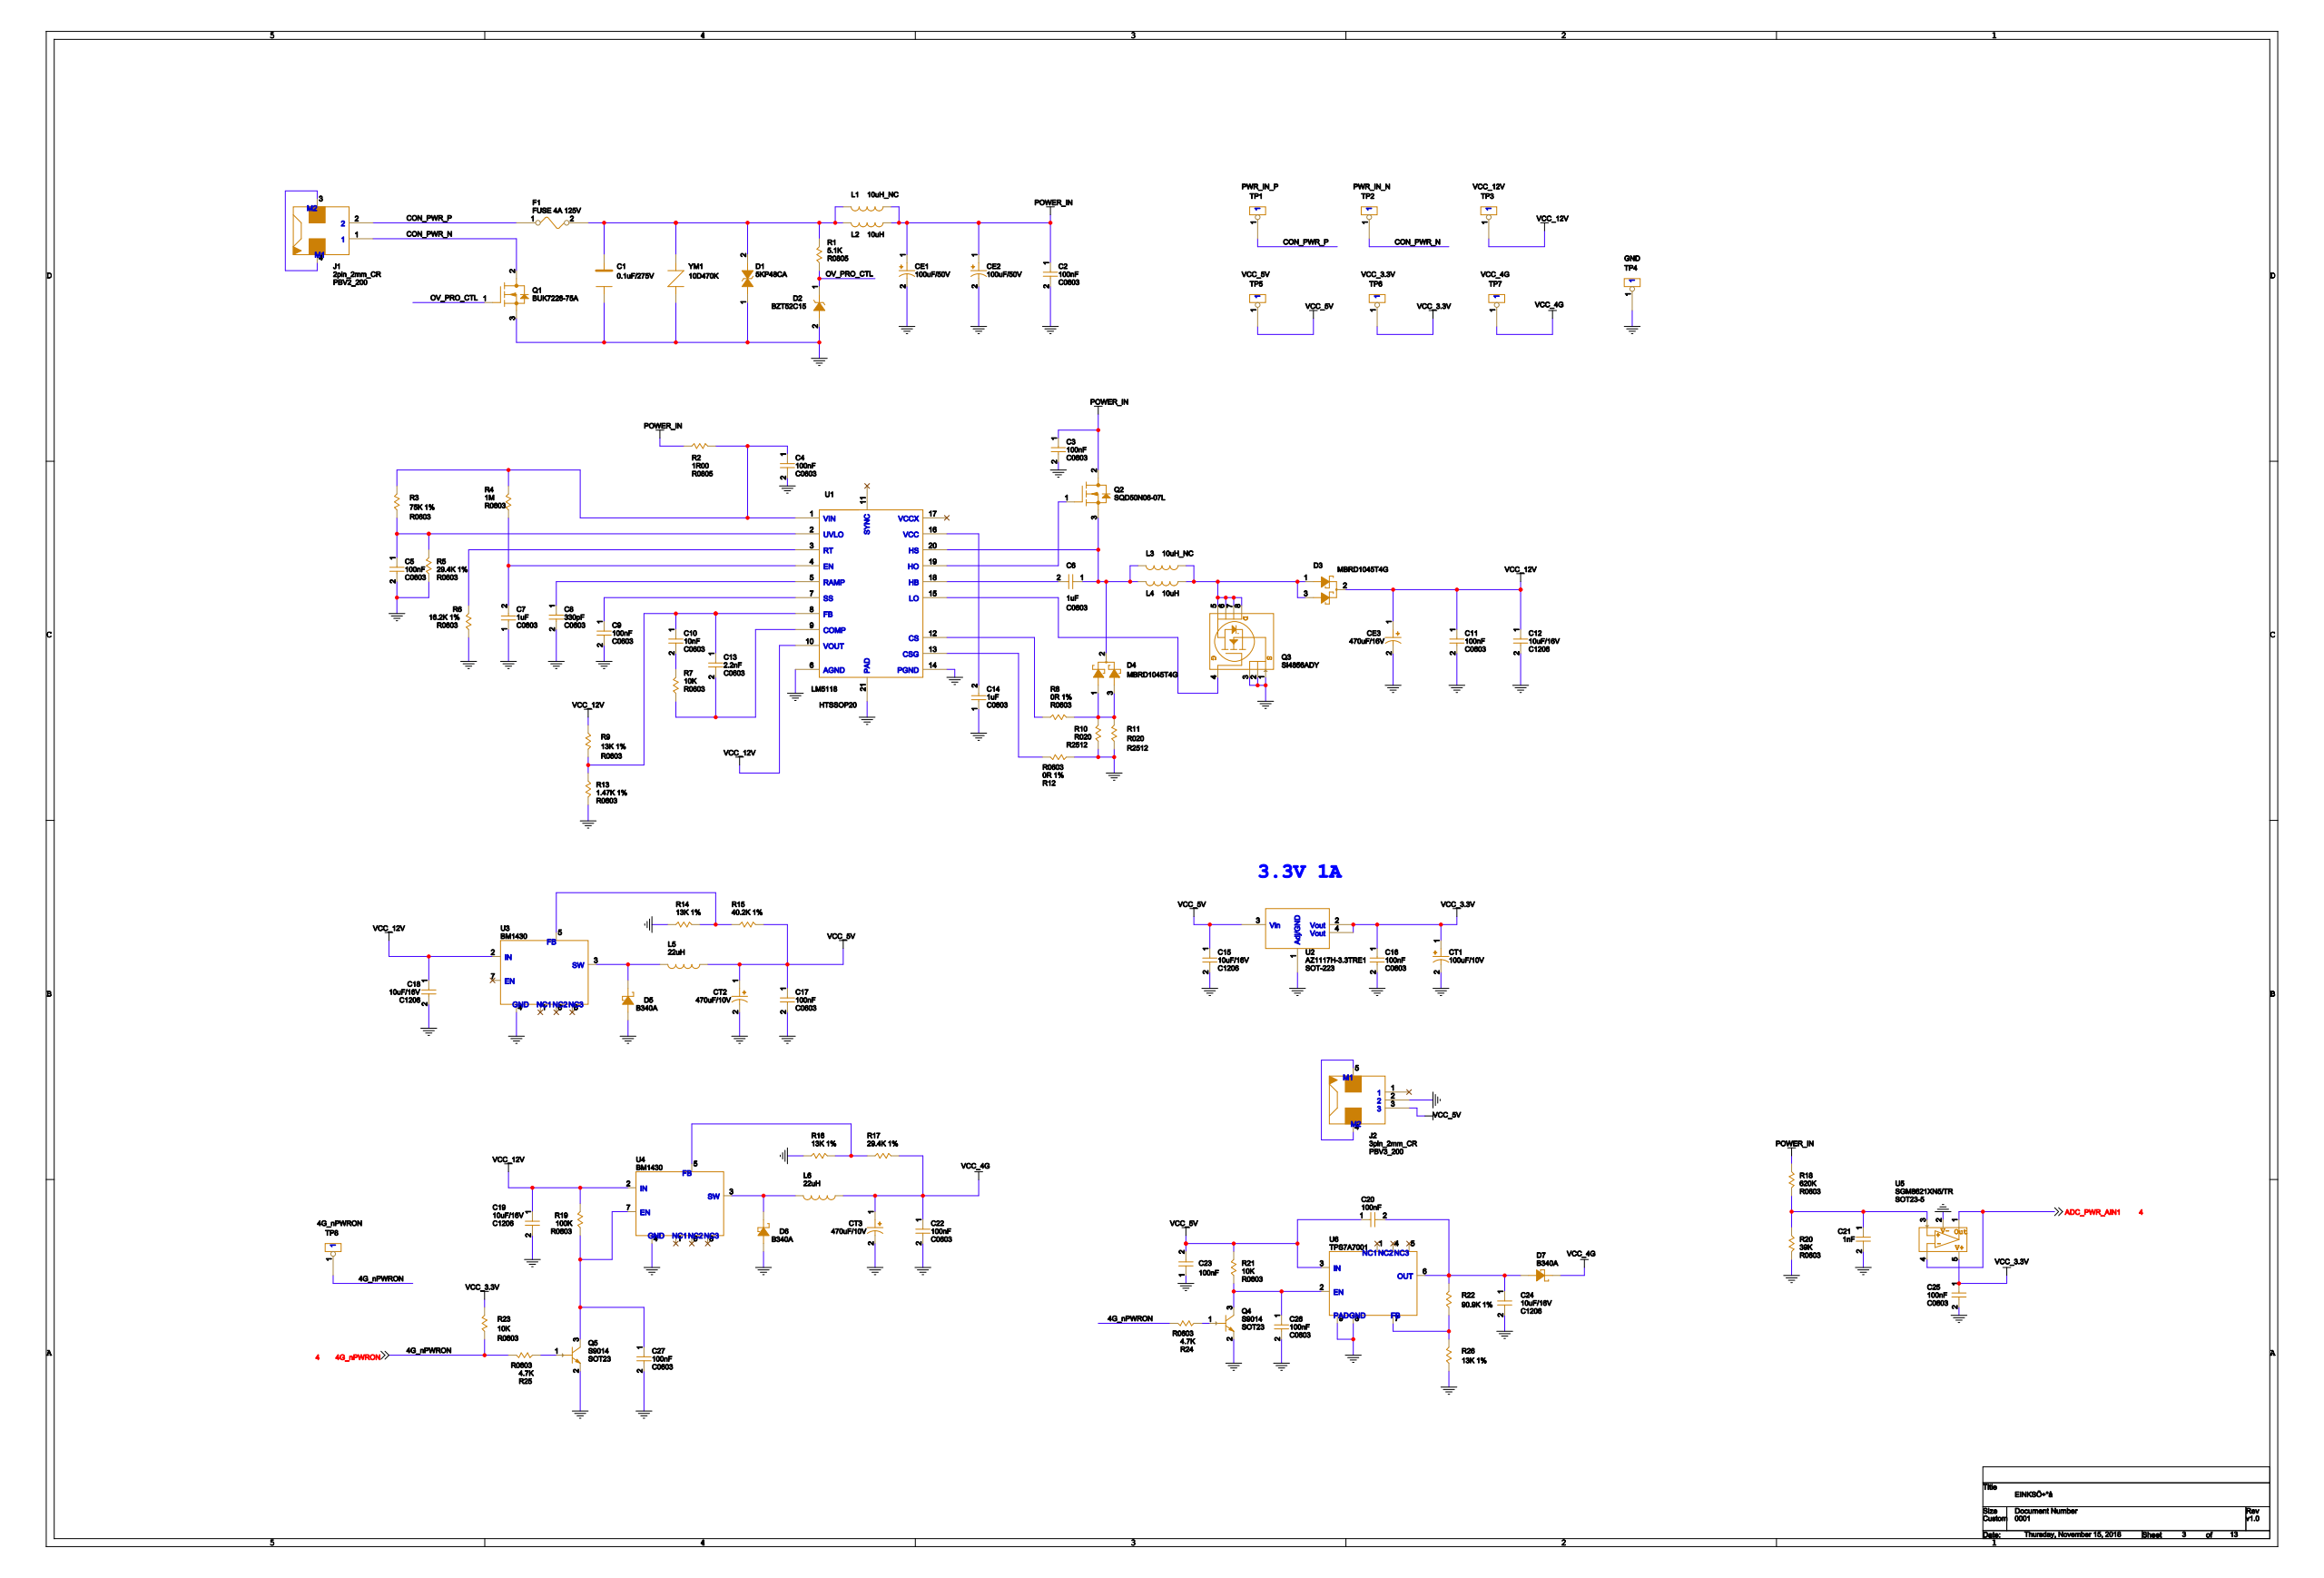Circuit board | Cadence Allegro | 609 parts | 409 nets | one sheet of the schematic
Parts on this sheet (reference | value | footprint):
C1 | 0.1uF/275V | C_18X6L
C2 | 100nF | C0603
C3 | 100nF | C0603
C4 | 100nF | C0603
C5 | 100nF | C0603
C6 | 1uF | C0603
C7 | 1uF | C0603
C8 | 330pF | C0603
C9 | 100nF | C0603
C10 | 10nF | C0603
C11 | 100nF | C0603
C12 | 10uF/16V | C1206
C13 | 2.2nF | C0603
C14 | 1uF | C0603
C15 | 10uF/16V | C1206
C16 | 100nF | C0603
C17 | 100nF | C0603
C18 | 10uF/16V | C1206
C19 | 10uF/16V | C1206
C20 | 100nF | C0603
C21 | 1nF | C0603
C22 | 100nF | C0603
C23 | 100nF | C0603
C24 | 10uF/16V | C1206
C25 | 100nF | C0603
C26 | 100nF | C0603
C27 | 100nF | C0603
CE1 | 100uF/50V | CE8X11D5P3D5L
CE2 | 100uF/50V | CE8X11D5P3D5L
CE3 | 470uF/16V | CE8X11D5P3D5L
CT1 | 100uF/10V | B_CASE
CT2 | 470uF/10V | E_CASE
CT3 | 470uF/10V | E_CASE
D1 | 5KP48CA | 5KP48A
D2 | BZT52C15 | SOD-123FL
D3 | MBRD1045T4G | SOT428
D4 | MBRD1045T4G | SOT428
D5 | B340A | DO-214AA
D6 | B340A | DO-214AA
D7 | B340A | DO-214AA
F1 | FUSE 4A 125V | F_065
J1 | 2pin_2mm_CR | PBV2_200
J2 | 3pin_2mm_CR | PBV3_200
L1 | 10uH_NC | IND_VLS6045
L2 | 10uH | L_C150_C50
L3 | 10uH_NC | IND_VLS6045
L4 | 10uH | L_C150_C50
L5 | 22uH | IND_VLS6045
L6 | 22uH | IND_VLS6045
Q1 | BUK7226-75A | SOT428
Q2 | SQD50N06-07L | SOT428
Q3 | SI4856ADY | SOIC8
Q4 | S9014 | SOT23
Q5 | S9014 | SOT23
R1 | 5.1K | R0805
R2 | 1R00 | R0805
R4 | 1M | R0603
R6 | 16.2K 1% | R0603
R7 | 10K | R0603
R8 | 0R 1% | R0603
R9 | 13K 1% | R0603
R10 | R020 | R2512
R11 | R020 | R2512
R15 | 40.2K 1% | R0603
R16 | 13K 1% | R0603
R17 | 29.4K 1% | R0603
R18 | 620K | R0603
R19 | 100K | R0603
R20 | 39K | R0603
R21 | 10K | R0603
R22 | 90.9K 1% | R0603
R23 | 10K | R0603
R24 | 4.7K | R0603
R25 | 4.7K | R0603
R26 | 13K 1% | R0603
TP1 | PWR_IN_P | TP_50
TP2 | PWR_IN_N | TP_50
TP3 | VCC_12V | TP_50
TP4 | GND | TP_50
TP5 | VCC_5V | TP_50
TP6 | VCC_3.3V | TP_50
TP7 | VCC_4G | TP_50
TP8 | 4G_nPWRON | TP_50
U1 | LM5118 | HTSSOP20
U2 | AZ1117H-3.3TRE1 | SOT-223
U3 | BM1430 | SOIC8
U4 | BM1430 | SOIC8
U5 | SGM8621XN5/TR | SOT23-5
U6 | TPS7A7001 | HSOIC8
YM1 | 10D470K | CON_2X7MML
Nets of these parts (net: part-pin ...):
GND: C1-2 C2-2 C3-2 C4-2 C5-2 C7-1 C8-2 C9-2 C11-2 C12-2 C14-1 C15-2 C16-2 C17-2 C18-2 C19-2 C21-2 C22-2 C23-1 C24-2 C25-2 C26-2 C27-2 CE1-2 CE2-2 CE3-2 CT1-2 CT2-2 CT3-2 D1-1 D2-2 D5-1 D6-1 J2-2 Q1-3 Q3-1 Q3-2 Q3-3 Q4-2 Q5-2 R6-1 R10-1 R11-1 R16-1 R20-2 R26-1 TP4-1 U1-6 U1-14 U1-21 U2-1 U3-4 U4-4 U5-2 U6-8 U6-9 YM1-1
N28604991: C1-1 D1-2 F1-2 L1-2 L2-2 R1-2 YM1-2
POWER_IN: C2-1 C3-1 CE1-1 CE2-1 L1-1 L2-1 Q2-2 R2-2 R18-2
VCC_12V: C11-1 C12-1 C18-1 C19-1 CE3-1 D3-2 R9-1 R19-2 TP3-1 U1-10 U3-2 U4-2
VCC_3.3V: C16-1 C25-1 CT1-1 R23-2 TP6-1 U2-2 U2-4 U5-5
VCC_5V: C15-1 C17-1 C20-1 C23-2 CT2-1 J2-3 L5-1 R15-2 R21-2 TP5-1 U2-3 U6-3
VCC_4G: C22-1 CT3-1 D7-2 L6-1 R17-2 TP7-1
CON_PWR_P: F1-1 J1-2 TP1-1
CON_PWR_N: J1-1 Q1-2 TP2-1
N28625797: J1-3 J1-4
N28624762: J2-4 J2-5
4G_NPWRON: R23-1 R24-2 R25-2 TP8-1
N28605021: D3-1 D3-3 L3-1 L4-1 Q3-5 Q3-6 Q3-7 Q3-8
N28605022: C6-1 D4-2 L3-2 L4-2 Q2-3 U1-20
OV_PRO_CTL: D2-1 Q1-1 R1-1
N28605217: C21-1 R18-1 R20-1 U5-3
N28605116: R15-1 U3-5
ADC_PWR_AIN1: U5-1 U5-4
N28623164: R22-1 R26-2 U6-7
N28623166: C20-2 C24-1 D7-1 R22-2 U6-6
N28623202: C26-1 Q4-3 R21-1 U6-2
N28605064: C8-1 U1-5
N28605069: C10-1 C13-1 R9-2 U1-8
N28605072: C13-2 R7-1 U1-9
N28605061: C7-2 R4-1 U1-4
N28605048: C14-2 U1-16
N28605040: C6-2 U1-18
N28605010: D4-1 D4-3 R8-2 R10-2 R11-2
N28605127: D6-2 L6-2 U4-3
N28605105: D5-2 L5-2 U3-3
N28605024: Q2-1 U1-19
N28605015: Q3-4 U1-15
N28605017: C4-1 R2-1 R4-2 U1-1
N28605204: C10-2 R7-2
N28623331: Q4-1 R24-1
N28605154: Q5-1 R25-1
N28605013: U1-13
N28605011: R8-1 U1-12
N28605156: C27-1 Q5-3 R19-1 U4-7
N28605052: C5-1 U1-2
N28605135: R16-2 R17-1 U4-5
N28605059: R6-2 U1-3
N28605066: C9-1 U1-7